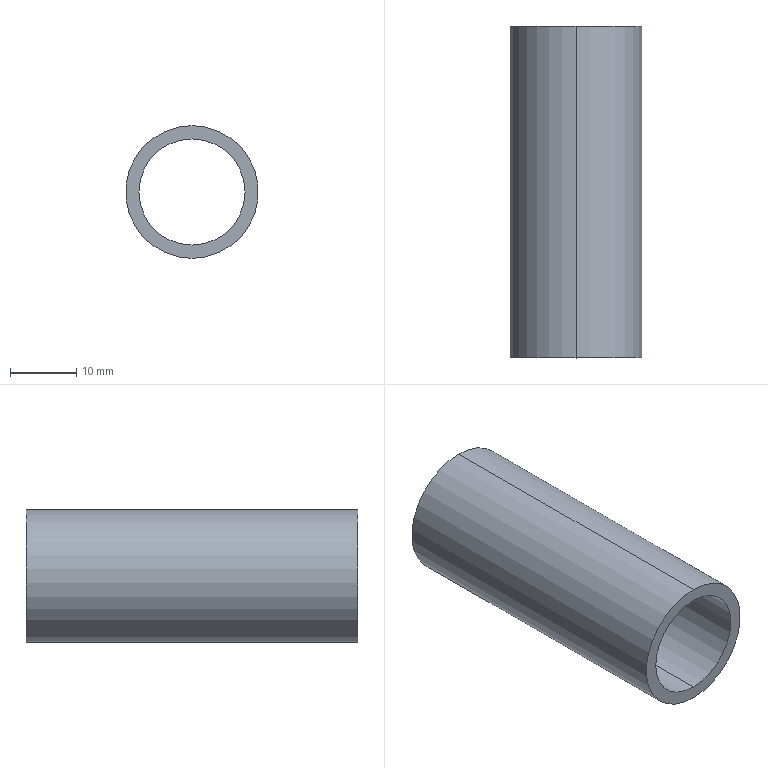Part | SolidWorks | features Extrusion 1 | 1 solid | 6 faces | box 20 x 50 x 20 mm | volume 5655 mm3 | cylinder 4 | plane 2 | commonest cylinder face diameters 16 x2 20 x2
STEP:
#1=CARTESIAN_POINT('',(0.,50.,-8.));
#2=VERTEX_POINT('',#1);
#3=CARTESIAN_POINT('',(0.,50.,8.));
#4=VERTEX_POINT('',#3);
#5=CARTESIAN_POINT('',(0.,50.,0.));
#6=DIRECTION('',(0.,1.,0.));
#7=DIRECTION('',(0.,0.,1.));
#8=AXIS2_PLACEMENT_3D('',#5,#6,#7);
#9=CIRCLE('',#8,8.);
#10=EDGE_CURVE('',#2,#4,#9,.T.);
#11=ORIENTED_EDGE('',*,*,#10,.T.);
#12=CARTESIAN_POINT('',(0.,0.,8.));
#13=VERTEX_POINT('',#12);
#14=CARTESIAN_POINT('',(0.,50.,8.));
#15=DIRECTION('',(0.,-1.,0.));
#16=VECTOR('',#15,1000.);
#17=LINE('',#14,#16);
#18=EDGE_CURVE('',#4,#13,#17,.T.);
#19=ORIENTED_EDGE('',*,*,#18,.T.);
#20=CARTESIAN_POINT('',(0.,0.,-8.));
#21=VERTEX_POINT('',#20);
#22=CARTESIAN_POINT('',(0.,0.,0.));
#23=DIRECTION('',(0.,1.,0.));
#24=DIRECTION('',(0.,0.,1.));
#25=AXIS2_PLACEMENT_3D('',#22,#23,#24);
#26=CIRCLE('',#25,8.);
#27=EDGE_CURVE('',#21,#13,#26,.T.);
#28=ORIENTED_EDGE('',*,*,#27,.F.);
#29=CARTESIAN_POINT('',(0.,50.,-8.));
#30=DIRECTION('',(0.,-1.,0.));
#31=VECTOR('',#30,1000.);
#32=LINE('',#29,#31);
#33=EDGE_CURVE('',#2,#21,#32,.T.);
#34=ORIENTED_EDGE('',*,*,#33,.F.);
#35=EDGE_LOOP('',(#11,#19,#28,#34));
#36=FACE_OUTER_BOUND('',#35,.T.);
#37=CARTESIAN_POINT('',(0.,50.,0.));
#38=DIRECTION('',(0.,-1.,0.));
#39=DIRECTION('',(0.,0.,-1.));
#40=AXIS2_PLACEMENT_3D('',#37,#38,#39);
#41=CYLINDRICAL_SURFACE('',#40,8.);
#42=ADVANCED_FACE('',(#36),#41,.F.);
#43=CARTESIAN_POINT('',(0.,50.,10.));
#44=VERTEX_POINT('',#43);
#45=CARTESIAN_POINT('',(0.,50.,-10.));
#46=VERTEX_POINT('',#45);
#47=CARTESIAN_POINT('',(0.,50.,0.));
#48=DIRECTION('',(0.,1.,0.));
#49=DIRECTION('',(0.,0.,1.));
#50=AXIS2_PLACEMENT_3D('',#47,#48,#49);
#51=CIRCLE('',#50,10.);
#52=EDGE_CURVE('',#44,#46,#51,.T.);
#53=ORIENTED_EDGE('',*,*,#52,.F.);
#54=CARTESIAN_POINT('',(0.,0.,10.));
#55=VERTEX_POINT('',#54);
#56=CARTESIAN_POINT('',(0.,50.,10.));
#57=DIRECTION('',(0.,-1.,0.));
#58=VECTOR('',#57,1000.);
#59=LINE('',#56,#58);
#60=EDGE_CURVE('',#44,#55,#59,.T.);
#61=ORIENTED_EDGE('',*,*,#60,.T.);
#62=CARTESIAN_POINT('',(0.,0.,-10.));
#63=VERTEX_POINT('',#62);
#64=CARTESIAN_POINT('',(0.,0.,0.));
#65=DIRECTION('',(0.,1.,0.));
#66=DIRECTION('',(0.,0.,1.));
#67=AXIS2_PLACEMENT_3D('',#64,#65,#66);
#68=CIRCLE('',#67,10.);
#69=EDGE_CURVE('',#55,#63,#68,.T.);
#70=ORIENTED_EDGE('',*,*,#69,.T.);
#71=CARTESIAN_POINT('',(0.,50.,-10.));
#72=DIRECTION('',(0.,-1.,0.));
#73=VECTOR('',#72,1000.);
#74=LINE('',#71,#73);
#75=EDGE_CURVE('',#46,#63,#74,.T.);
#76=ORIENTED_EDGE('',*,*,#75,.F.);
#77=EDGE_LOOP('',(#53,#61,#70,#76));
#78=FACE_OUTER_BOUND('',#77,.T.);
#79=CARTESIAN_POINT('',(0.,50.,0.));
#80=DIRECTION('',(0.,-1.,0.));
#81=DIRECTION('',(0.,0.,-1.));
#82=AXIS2_PLACEMENT_3D('',#79,#80,#81);
#83=CYLINDRICAL_SURFACE('',#82,10.);
#84=ADVANCED_FACE('',(#78),#83,.T.);
#85=CARTESIAN_POINT('',(0.,50.,0.));
#86=DIRECTION('',(0.,1.,0.));
#87=DIRECTION('',(0.,0.,1.));
#88=AXIS2_PLACEMENT_3D('',#85,#86,#87);
#89=CIRCLE('',#88,10.);
#90=EDGE_CURVE('',#46,#44,#89,.T.);
#91=ORIENTED_EDGE('',*,*,#90,.T.);
#92=ORIENTED_EDGE('',*,*,#52,.T.);
#93=EDGE_LOOP('',(#91,#92));
#94=FACE_OUTER_BOUND('',#93,.T.);
#95=ORIENTED_EDGE('',*,*,#10,.F.);
#96=CARTESIAN_POINT('',(0.,50.,0.));
#97=DIRECTION('',(0.,1.,0.));
#98=DIRECTION('',(0.,0.,1.));
#99=AXIS2_PLACEMENT_3D('',#96,#97,#98);
#100=CIRCLE('',#99,8.);
#101=EDGE_CURVE('',#4,#2,#100,.T.);
#102=ORIENTED_EDGE('',*,*,#101,.F.);
#103=EDGE_LOOP('',(#95,#102));
#104=FACE_BOUND('',#103,.T.);
#105=CARTESIAN_POINT('',(0.,50.,0.));
#106=DIRECTION('',(0.,1.,0.));
#107=DIRECTION('',(0.,0.,1.));
#108=AXIS2_PLACEMENT_3D('',#105,#106,#107);
#109=PLANE('',#108);
#110=ADVANCED_FACE('',(#94,#104),#109,.T.);
#111=CARTESIAN_POINT('',(0.,0.,0.));
#112=DIRECTION('',(0.,1.,0.));
#113=DIRECTION('',(0.,0.,1.));
#114=AXIS2_PLACEMENT_3D('',#111,#112,#113);
#115=CIRCLE('',#114,10.);
#116=EDGE_CURVE('',#63,#55,#115,.T.);
#117=ORIENTED_EDGE('',*,*,#116,.F.);
#118=ORIENTED_EDGE('',*,*,#69,.F.);
#119=EDGE_LOOP('',(#117,#118));
#120=FACE_OUTER_BOUND('',#119,.T.);
#121=ORIENTED_EDGE('',*,*,#27,.T.);
#122=CARTESIAN_POINT('',(0.,0.,0.));
#123=DIRECTION('',(0.,1.,0.));
#124=DIRECTION('',(0.,0.,1.));
#125=AXIS2_PLACEMENT_3D('',#122,#123,#124);
#126=CIRCLE('',#125,8.);
#127=EDGE_CURVE('',#13,#21,#126,.T.);
#128=ORIENTED_EDGE('',*,*,#127,.T.);
#129=EDGE_LOOP('',(#121,#128));
#130=FACE_BOUND('',#129,.T.);
#131=CARTESIAN_POINT('',(0.,0.,0.));
#132=DIRECTION('',(0.,1.,0.));
#133=DIRECTION('',(0.,0.,1.));
#134=AXIS2_PLACEMENT_3D('',#131,#132,#133);
#135=PLANE('',#134);
#136=ADVANCED_FACE('',(#120,#130),#135,.F.);
#137=ORIENTED_EDGE('',*,*,#60,.F.);
#138=ORIENTED_EDGE('',*,*,#90,.F.);
#139=ORIENTED_EDGE('',*,*,#75,.T.);
#140=ORIENTED_EDGE('',*,*,#116,.T.);
#141=EDGE_LOOP('',(#137,#138,#139,#140));
#142=FACE_OUTER_BOUND('',#141,.T.);
#143=CARTESIAN_POINT('',(0.,50.,0.));
#144=DIRECTION('',(0.,-1.,0.));
#145=DIRECTION('',(0.,0.,-1.));
#146=AXIS2_PLACEMENT_3D('',#143,#144,#145);
#147=CYLINDRICAL_SURFACE('',#146,10.);
#148=ADVANCED_FACE('',(#142),#147,.T.);
#149=ORIENTED_EDGE('',*,*,#18,.F.);
#150=ORIENTED_EDGE('',*,*,#101,.T.);
#151=ORIENTED_EDGE('',*,*,#33,.T.);
#152=ORIENTED_EDGE('',*,*,#127,.F.);
#153=EDGE_LOOP('',(#149,#150,#151,#152));
#154=FACE_OUTER_BOUND('',#153,.T.);
#155=CARTESIAN_POINT('',(0.,50.,0.));
#156=DIRECTION('',(0.,-1.,0.));
#157=DIRECTION('',(0.,0.,-1.));
#158=AXIS2_PLACEMENT_3D('',#155,#156,#157);
#159=CYLINDRICAL_SURFACE('',#158,8.);
#160=ADVANCED_FACE('',(#154),#159,.F.);
#161=CLOSED_SHELL('',(#42,#84,#110,#136,#148,#160));
#162=MANIFOLD_SOLID_BREP('',#161);
#163=CARTESIAN_POINT('',(0.,0.,0.));
#164=DIRECTION('',(0.,0.,1.));
#165=DIRECTION('',(1.,0.,0.));
#166=AXIS2_PLACEMENT_3D('',#163,#164,#165);
#167=(LENGTH_UNIT()NAMED_UNIT(*)SI_UNIT(.MILLI.,.METRE.));
#168=UNCERTAINTY_MEASURE_WITH_UNIT(LENGTH_MEASURE(0.00001),#167,'','');
#169=(NAMED_UNIT(*)PLANE_ANGLE_UNIT()SI_UNIT($,.RADIAN.));
#170=(NAMED_UNIT(*)SI_UNIT($,.STERADIAN.)SOLID_ANGLE_UNIT());
#171=(GEOMETRIC_REPRESENTATION_CONTEXT(3)GLOBAL_UNCERTAINTY_ASSIGNED_CONTEXT((#168))GLOBAL_UNIT_ASSIGNED_CONTEXT((#167,#169,#170))REPRESENTATION_CONTEXT('',''));
#172=ADVANCED_BREP_SHAPE_REPRESENTATION('',(#162,#166),#171);